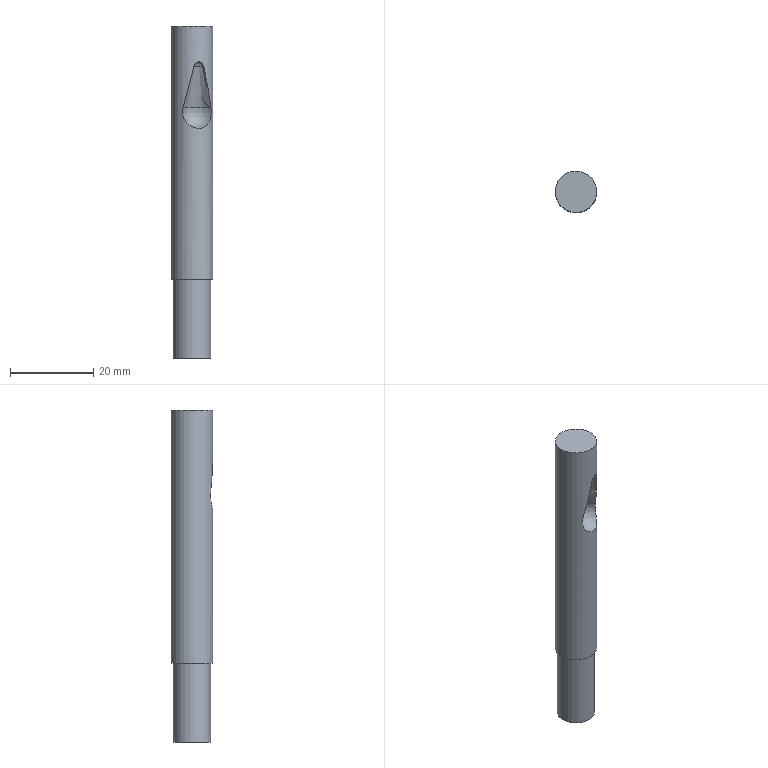Part | NX | features solid 2 | 1 solid | 8 faces | volume 5822 mm3 | plane 3 | cylinder 2 | sphere 2 | cone 1 | commonest cylinder face diameters 9 x1 10 x1
STEP:
#1=CARTESIAN_POINT('',(-1359.448,364.514,104.333));
#2=VERTEX_POINT('',#1);
#3=CARTESIAN_POINT('',(-1361.144,362.478,114.333));
#4=VERTEX_POINT('',#3);
#5=CARTESIAN_POINT('',(-1359.448,364.514,104.333));
#6=CARTESIAN_POINT('',(-1359.833,363.666,107.658));
#7=CARTESIAN_POINT('',(-1360.43,362.974,110.992));
#8=CARTESIAN_POINT('',(-1361.144,362.478,114.333));
#9=B_SPLINE_CURVE_WITH_KNOTS('',3,(#5,#6,#7,#8),.UNSPECIFIED.,.F.,.F.,(4,4),(0.000000207,0.01035),.UNSPECIFIED.);
#10=EDGE_CURVE('',#2,#4,#9,.T.);
#11=ORIENTED_EDGE('',*,*,#10,.F.);
#12=CARTESIAN_POINT('',(-1366.158,362.071,104.333));
#13=VERTEX_POINT('',#12);
#14=CARTESIAN_POINT('',(-1366.158,362.071,104.333));
#15=CARTESIAN_POINT('',(-1366.309,362.143,103.737));
#16=CARTESIAN_POINT('',(-1366.334,362.157,102.48));
#17=CARTESIAN_POINT('',(-1365.562,361.783,100.792));
#18=CARTESIAN_POINT('',(-1364.098,361.486,99.625));
#19=CARTESIAN_POINT('',(-1362.258,361.765,99.188));
#20=CARTESIAN_POINT('',(-1360.651,362.737,99.621));
#21=CARTESIAN_POINT('',(-1359.719,363.91,100.792));
#22=CARTESIAN_POINT('',(-1359.368,364.692,102.477));
#23=CARTESIAN_POINT('',(-1359.378,364.666,103.737));
#24=CARTESIAN_POINT('',(-1359.448,364.514,104.333));
#25=B_SPLINE_CURVE_WITH_KNOTS('',3,(#14,#15,#16,#17,#18,#19,#20,#21,#22,#23,#24),.UNSPECIFIED.,.F.,.F.,(4,1,1,1,1,1,1,1,4),(0.000000205,0.001831,0.003662,0.005493,0.007324,0.009155,0.01099,0.01282,0.01465),.UNSPECIFIED.);
#26=EDGE_CURVE('',#13,#2,#25,.T.);
#27=ORIENTED_EDGE('',*,*,#26,.F.);
#28=CARTESIAN_POINT('',(-1363.55,361.602,114.333));
#29=VERTEX_POINT('',#28);
#30=CARTESIAN_POINT('',(-1363.55,361.602,114.333));
#31=CARTESIAN_POINT('',(-1364.417,361.523,110.991));
#32=CARTESIAN_POINT('',(-1365.318,361.669,107.66));
#33=CARTESIAN_POINT('',(-1366.158,362.071,104.333));
#34=B_SPLINE_CURVE_WITH_KNOTS('',3,(#30,#31,#32,#33),.UNSPECIFIED.,.F.,.F.,(4,4),(0.000000207,0.01036),.UNSPECIFIED.);
#35=EDGE_CURVE('',#29,#13,#34,.T.);
#36=ORIENTED_EDGE('',*,*,#35,.F.);
#37=CARTESIAN_POINT('',(-1361.144,362.478,114.333));
#38=CARTESIAN_POINT('',(-1361.266,362.392,114.906));
#39=CARTESIAN_POINT('',(-1362.244,361.763,115.76));
#40=CARTESIAN_POINT('',(-1363.401,361.615,114.906));
#41=CARTESIAN_POINT('',(-1363.55,361.602,114.333));
#42=B_SPLINE_CURVE_WITH_KNOTS('',3,(#37,#38,#39,#40,#41),.UNSPECIFIED.,.F.,.F.,(4,1,4),(0.000000204,0.001751,0.003502),.UNSPECIFIED.);
#43=EDGE_CURVE('',#4,#29,#42,.T.);
#44=ORIENTED_EDGE('',*,*,#43,.F.);
#45=EDGE_LOOP('',(#11,#27,#36,#44));
#46=FACE_BOUND('',#45,.T.);
#47=CARTESIAN_POINT('',(-1359.302,368.292,124.));
#48=VERTEX_POINT('',#47);
#49=CARTESIAN_POINT('',(-1364.,366.582,124.));
#50=DIRECTION('',(0.,0.,-1.));
#51=DIRECTION('',(0.9397,0.342,0.));
#52=AXIS2_PLACEMENT_3D('',#49,#50,#51);
#53=CIRCLE('',#52,5.);
#54=EDGE_CURVE('',#48,#48,#53,.T.);
#55=ORIENTED_EDGE('',*,*,#54,.T.);
#56=EDGE_LOOP('',(#55));
#57=FACE_BOUND('',#56,.T.);
#58=CARTESIAN_POINT('',(-1359.302,368.292,63.));
#59=VERTEX_POINT('',#58);
#60=CARTESIAN_POINT('',(-1364.,366.582,63.));
#61=DIRECTION('',(0.,0.,-1.));
#62=DIRECTION('',(0.9397,0.342,0.));
#63=AXIS2_PLACEMENT_3D('',#60,#61,#62);
#64=CIRCLE('',#63,5.);
#65=EDGE_CURVE('',#59,#59,#64,.T.);
#66=ORIENTED_EDGE('',*,*,#65,.F.);
#67=EDGE_LOOP('',(#66));
#68=FACE_BOUND('',#67,.T.);
#69=CARTESIAN_POINT('',(-1364.,366.582,124.));
#70=DIRECTION('',(0.,0.,-1.));
#71=DIRECTION('',(-0.9397,-0.342,0.));
#72=AXIS2_PLACEMENT_3D('',#69,#70,#71);
#73=CYLINDRICAL_SURFACE('',#72,5.);
#74=ADVANCED_FACE('',(#46,#57,#68),#73,.T.);
#75=ORIENTED_EDGE('',*,*,#54,.F.);
#76=EDGE_LOOP('',(#75));
#77=FACE_BOUND('',#76,.T.);
#78=CARTESIAN_POINT('',(-1364.,366.582,124.));
#79=DIRECTION('',(0.,0.,1.));
#80=DIRECTION('',(0.9397,0.342,0.));
#81=AXIS2_PLACEMENT_3D('',#78,#79,#80);
#82=PLANE('',#81);
#83=ADVANCED_FACE('',(#77),#82,.T.);
#84=CARTESIAN_POINT('',(-1359.771,368.121,63.));
#85=VERTEX_POINT('',#84);
#86=CARTESIAN_POINT('',(-1364.,366.582,63.));
#87=DIRECTION('',(0.,0.,-1.));
#88=DIRECTION('',(0.9397,0.342,0.));
#89=AXIS2_PLACEMENT_3D('',#86,#87,#88);
#90=CIRCLE('',#89,4.5);
#91=EDGE_CURVE('',#85,#85,#90,.T.);
#92=ORIENTED_EDGE('',*,*,#91,.F.);
#93=EDGE_LOOP('',(#92));
#94=FACE_BOUND('',#93,.T.);
#95=ORIENTED_EDGE('',*,*,#65,.T.);
#96=EDGE_LOOP('',(#95));
#97=FACE_BOUND('',#96,.T.);
#98=CARTESIAN_POINT('',(-1364.,366.582,63.));
#99=DIRECTION('',(0.,0.,1.));
#100=DIRECTION('',(0.9397,0.342,0.));
#101=AXIS2_PLACEMENT_3D('',#98,#99,#100);
#102=PLANE('',#101);
#103=ADVANCED_FACE('',(#94,#97),#102,.F.);
#104=CARTESIAN_POINT('',(-1359.771,368.121,44.));
#105=VERTEX_POINT('',#104);
#106=CARTESIAN_POINT('',(-1364.,366.582,44.));
#107=DIRECTION('',(0.,0.,-1.));
#108=DIRECTION('',(0.9397,0.342,0.));
#109=AXIS2_PLACEMENT_3D('',#106,#107,#108);
#110=CIRCLE('',#109,4.5);
#111=EDGE_CURVE('',#105,#105,#110,.T.);
#112=ORIENTED_EDGE('',*,*,#111,.F.);
#113=EDGE_LOOP('',(#112));
#114=FACE_BOUND('',#113,.T.);
#115=ORIENTED_EDGE('',*,*,#91,.T.);
#116=EDGE_LOOP('',(#115));
#117=FACE_BOUND('',#116,.T.);
#118=CARTESIAN_POINT('',(-1364.,366.582,44.));
#119=DIRECTION('',(0.,0.,1.));
#120=DIRECTION('',(0.9397,0.342,0.));
#121=AXIS2_PLACEMENT_3D('',#118,#119,#120);
#122=CYLINDRICAL_SURFACE('',#121,4.5);
#123=ADVANCED_FACE('',(#114,#117),#122,.T.);
#124=ORIENTED_EDGE('',*,*,#111,.T.);
#125=EDGE_LOOP('',(#124));
#126=FACE_BOUND('',#125,.T.);
#127=CARTESIAN_POINT('',(-1364.,366.582,44.));
#128=DIRECTION('',(0.,0.,1.));
#129=DIRECTION('',(0.9397,0.342,0.));
#130=AXIS2_PLACEMENT_3D('',#127,#128,#129);
#131=PLANE('',#130);
#132=ADVANCED_FACE('',(#126),#131,.F.);
#133=CARTESIAN_POINT('',(-1362.29,361.883,104.333));
#134=DIRECTION('',(0.,0.,1.));
#135=DIRECTION('',(-0.9397,-0.342,0.));
#136=AXIS2_PLACEMENT_3D('',#133,#134,#135);
#137=CIRCLE('',#136,3.873);
#138=EDGE_CURVE('',#2,#13,#137,.T.);
#139=ORIENTED_EDGE('',*,*,#138,.T.);
#140=ORIENTED_EDGE('',*,*,#26,.T.);
#141=EDGE_LOOP('',(#139,#140));
#142=FACE_BOUND('',#141,.T.);
#143=CARTESIAN_POINT('',(-1362.29,361.883,103.333));
#144=DIRECTION('',(0.,0.,-1.));
#145=DIRECTION('',(-0.9397,-0.342,0.));
#146=AXIS2_PLACEMENT_3D('',#143,#144,#145);
#147=SPHERICAL_SURFACE('',#146,4.);
#148=ADVANCED_FACE('',(#142),#147,.F.);
#149=CARTESIAN_POINT('',(-1362.29,361.883,114.333));
#150=DIRECTION('',(0.,0.,1.));
#151=DIRECTION('',(-0.9397,-0.342,0.));
#152=AXIS2_PLACEMENT_3D('',#149,#150,#151);
#153=CIRCLE('',#152,1.291);
#154=EDGE_CURVE('',#4,#29,#153,.T.);
#155=ORIENTED_EDGE('',*,*,#154,.T.);
#156=ORIENTED_EDGE('',*,*,#35,.T.);
#157=ORIENTED_EDGE('',*,*,#138,.F.);
#158=ORIENTED_EDGE('',*,*,#10,.T.);
#159=EDGE_LOOP('',(#155,#156,#157,#158));
#160=FACE_BOUND('',#159,.T.);
#161=CARTESIAN_POINT('',(-1362.29,361.883,104.333));
#162=DIRECTION('',(0.,0.,-1.));
#163=DIRECTION('',(-0.9397,-0.342,0.));
#164=AXIS2_PLACEMENT_3D('',#161,#162,#163);
#165=CONICAL_SURFACE('',#164,3.873,0.2527);
#166=ADVANCED_FACE('',(#160),#165,.F.);
#167=ORIENTED_EDGE('',*,*,#154,.F.);
#168=ORIENTED_EDGE('',*,*,#43,.T.);
#169=EDGE_LOOP('',(#167,#168));
#170=FACE_BOUND('',#169,.T.);
#171=CARTESIAN_POINT('',(-1362.29,361.883,114.));
#172=DIRECTION('',(0.,0.,-1.));
#173=DIRECTION('',(0.9397,0.342,0.));
#174=AXIS2_PLACEMENT_3D('',#171,#172,#173);
#175=SPHERICAL_SURFACE('',#174,1.333);
#176=ADVANCED_FACE('',(#170),#175,.F.);
#177=CLOSED_SHELL('',(#74,#83,#103,#123,#132,#148,#166,#176));
#178=MANIFOLD_SOLID_BREP('',#177);
#179=(LENGTH_UNIT()NAMED_UNIT(*)SI_UNIT(.MILLI.,.METRE.));
#180=UNCERTAINTY_MEASURE_WITH_UNIT(LENGTH_MEASURE(0.0508),#179,'','');
#181=(NAMED_UNIT(*)PLANE_ANGLE_UNIT()SI_UNIT($,.RADIAN.));
#182=(NAMED_UNIT(*)SI_UNIT($,.STERADIAN.)SOLID_ANGLE_UNIT());
#183=(GEOMETRIC_REPRESENTATION_CONTEXT(3)GLOBAL_UNCERTAINTY_ASSIGNED_CONTEXT((#180))GLOBAL_UNIT_ASSIGNED_CONTEXT((#179,#181,#182))REPRESENTATION_CONTEXT('',''));
#184=ADVANCED_BREP_SHAPE_REPRESENTATION('',(#178),#183);